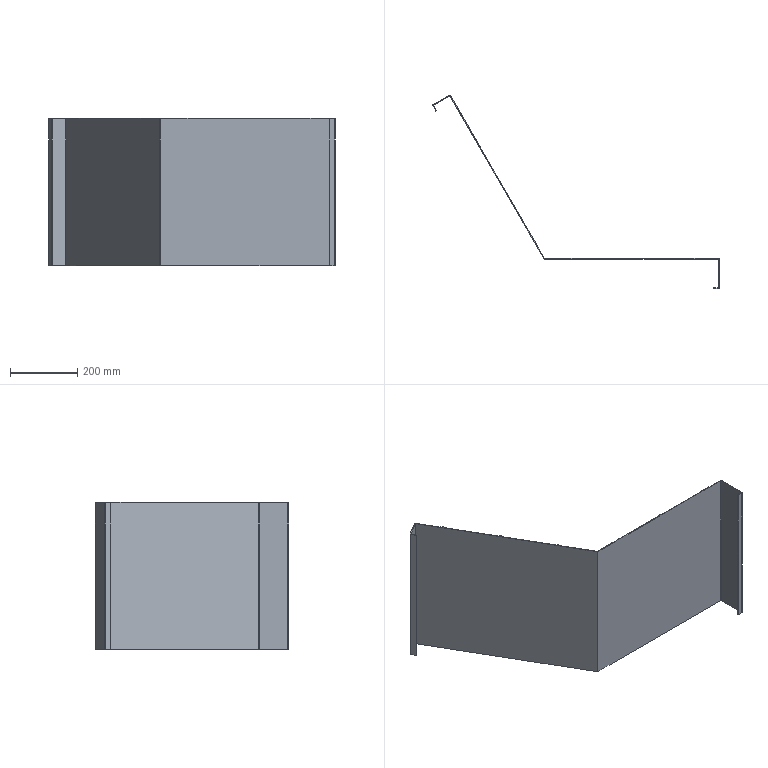Part | STEP file | zq002 | 1 solid | 52 faces | box 853.41 x 576.829 x 440 mm | volume 1105453 mm3 | plane 40 | cylinder 12 | commonest cylinder face diameters 1 x6 5 x6